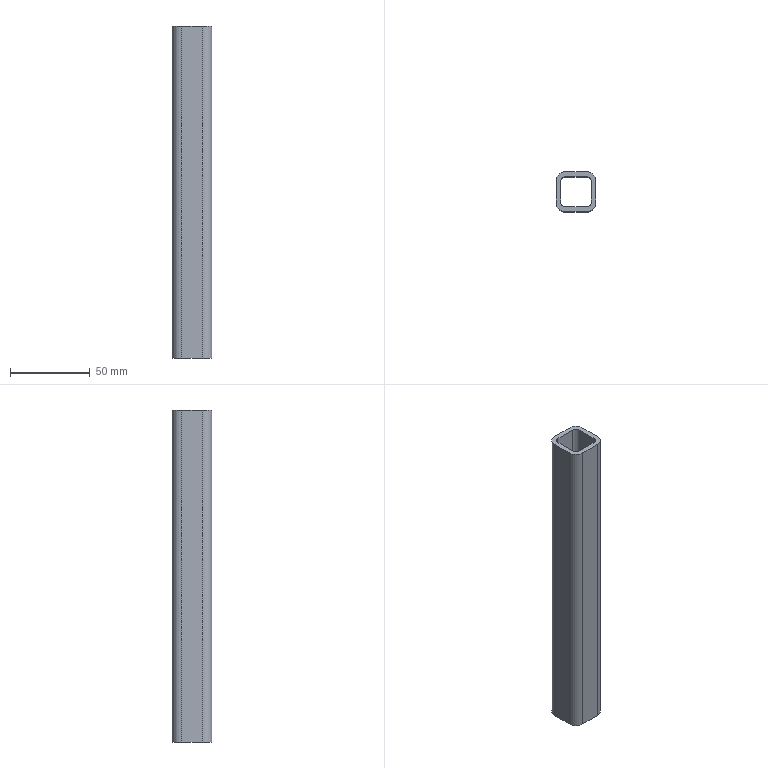Part | STEP file | ISO 10799-2 25x25x3 1784905468712 | 1 solid | 18 faces | box 25 x 25 x 208 mm | volume 50091 mm3 | plane 10 | cylinder 8 | commonest cylinder face diameters 6 x4 12 x4
STEP:
#1=CARTESIAN_POINT('',(-6.5,-9.5,208.));
#2=VERTEX_POINT('',#1);
#3=CARTESIAN_POINT('',(6.5,-9.5,208.));
#4=VERTEX_POINT('',#3);
#5=CARTESIAN_POINT('',(3.25,-9.5,208.));
#6=DIRECTION('',(1.,0.,0.));
#7=VECTOR('',#6,10.);
#8=LINE('',#5,#7);
#9=EDGE_CURVE('',#2,#4,#8,.T.);
#10=ORIENTED_EDGE('',*,*,#9,.T.);
#11=CARTESIAN_POINT('',(6.5,-9.5,0.));
#12=VERTEX_POINT('',#11);
#13=CARTESIAN_POINT('',(6.5,-9.5,0.));
#14=DIRECTION('',(0.,0.,1.));
#15=VECTOR('',#14,10.);
#16=LINE('',#13,#15);
#17=EDGE_CURVE('',#12,#4,#16,.T.);
#18=ORIENTED_EDGE('',*,*,#17,.F.);
#19=CARTESIAN_POINT('',(-6.5,-9.5,0.));
#20=VERTEX_POINT('',#19);
#21=CARTESIAN_POINT('',(3.25,-9.5,0.));
#22=DIRECTION('',(1.,0.,0.));
#23=VECTOR('',#22,10.);
#24=LINE('',#21,#23);
#25=EDGE_CURVE('',#20,#12,#24,.T.);
#26=ORIENTED_EDGE('',*,*,#25,.F.);
#27=CARTESIAN_POINT('',(-6.5,-9.5,0.));
#28=DIRECTION('',(0.,0.,1.));
#29=VECTOR('',#28,10.);
#30=LINE('',#27,#29);
#31=EDGE_CURVE('',#20,#2,#30,.T.);
#32=ORIENTED_EDGE('',*,*,#31,.T.);
#33=EDGE_LOOP('',(#10,#18,#26,#32));
#34=FACE_OUTER_BOUND('',#33,.T.);
#35=CARTESIAN_POINT('',(6.5,-9.5,0.));
#36=DIRECTION('',(0.,-1.,0.));
#37=DIRECTION('',(0.,0.,-1.));
#38=AXIS2_PLACEMENT_3D('',#35,#36,#37);
#39=PLANE('',#38);
#40=ADVANCED_FACE('',(#34),#39,.F.);
#41=CARTESIAN_POINT('',(9.5,-6.5,208.));
#42=VERTEX_POINT('',#41);
#43=CARTESIAN_POINT('',(6.5,-6.5,208.));
#44=DIRECTION('',(0.,0.,1.));
#45=DIRECTION('',(0.,1.,0.));
#46=AXIS2_PLACEMENT_3D('',#43,#44,#45);
#47=CIRCLE('',#46,3.);
#48=EDGE_CURVE('',#4,#42,#47,.T.);
#49=ORIENTED_EDGE('',*,*,#48,.T.);
#50=CARTESIAN_POINT('',(9.5,-6.5,0.));
#51=VERTEX_POINT('',#50);
#52=CARTESIAN_POINT('',(9.5,-6.5,0.));
#53=DIRECTION('',(0.,0.,1.));
#54=VECTOR('',#53,10.);
#55=LINE('',#52,#54);
#56=EDGE_CURVE('',#51,#42,#55,.T.);
#57=ORIENTED_EDGE('',*,*,#56,.F.);
#58=CARTESIAN_POINT('',(6.5,-6.5,0.));
#59=DIRECTION('',(0.,0.,1.));
#60=DIRECTION('',(0.,1.,0.));
#61=AXIS2_PLACEMENT_3D('',#58,#59,#60);
#62=CIRCLE('',#61,3.);
#63=EDGE_CURVE('',#12,#51,#62,.T.);
#64=ORIENTED_EDGE('',*,*,#63,.F.);
#65=ORIENTED_EDGE('',*,*,#17,.T.);
#66=EDGE_LOOP('',(#49,#57,#64,#65));
#67=FACE_OUTER_BOUND('',#66,.T.);
#68=CARTESIAN_POINT('',(6.5,-6.5,0.));
#69=DIRECTION('',(0.,0.,1.));
#70=DIRECTION('',(0.,1.,0.));
#71=AXIS2_PLACEMENT_3D('',#68,#69,#70);
#72=CYLINDRICAL_SURFACE('',#71,3.);
#73=ADVANCED_FACE('',(#67),#72,.F.);
#74=CARTESIAN_POINT('',(9.5,6.5,208.));
#75=VERTEX_POINT('',#74);
#76=CARTESIAN_POINT('',(9.5,3.25,208.));
#77=DIRECTION('',(0.,1.,0.));
#78=VECTOR('',#77,10.);
#79=LINE('',#76,#78);
#80=EDGE_CURVE('',#42,#75,#79,.T.);
#81=ORIENTED_EDGE('',*,*,#80,.T.);
#82=CARTESIAN_POINT('',(9.5,6.5,0.));
#83=VERTEX_POINT('',#82);
#84=CARTESIAN_POINT('',(9.5,6.5,0.));
#85=DIRECTION('',(0.,0.,1.));
#86=VECTOR('',#85,10.);
#87=LINE('',#84,#86);
#88=EDGE_CURVE('',#83,#75,#87,.T.);
#89=ORIENTED_EDGE('',*,*,#88,.F.);
#90=CARTESIAN_POINT('',(9.5,3.25,0.));
#91=DIRECTION('',(0.,1.,0.));
#92=VECTOR('',#91,10.);
#93=LINE('',#90,#92);
#94=EDGE_CURVE('',#51,#83,#93,.T.);
#95=ORIENTED_EDGE('',*,*,#94,.F.);
#96=ORIENTED_EDGE('',*,*,#56,.T.);
#97=EDGE_LOOP('',(#81,#89,#95,#96));
#98=FACE_OUTER_BOUND('',#97,.T.);
#99=CARTESIAN_POINT('',(9.5,6.5,0.));
#100=DIRECTION('',(1.,0.,0.));
#101=DIRECTION('',(0.,0.,-1.));
#102=AXIS2_PLACEMENT_3D('',#99,#100,#101);
#103=PLANE('',#102);
#104=ADVANCED_FACE('',(#98),#103,.F.);
#105=CARTESIAN_POINT('',(6.5,9.5,208.));
#106=VERTEX_POINT('',#105);
#107=CARTESIAN_POINT('',(6.5,6.5,208.));
#108=DIRECTION('',(0.,0.,1.));
#109=DIRECTION('',(-1.,0.,0.));
#110=AXIS2_PLACEMENT_3D('',#107,#108,#109);
#111=CIRCLE('',#110,3.);
#112=EDGE_CURVE('',#75,#106,#111,.T.);
#113=ORIENTED_EDGE('',*,*,#112,.T.);
#114=CARTESIAN_POINT('',(6.5,9.5,0.));
#115=VERTEX_POINT('',#114);
#116=CARTESIAN_POINT('',(6.5,9.5,0.));
#117=DIRECTION('',(0.,0.,1.));
#118=VECTOR('',#117,10.);
#119=LINE('',#116,#118);
#120=EDGE_CURVE('',#115,#106,#119,.T.);
#121=ORIENTED_EDGE('',*,*,#120,.F.);
#122=CARTESIAN_POINT('',(6.5,6.5,0.));
#123=DIRECTION('',(0.,0.,1.));
#124=DIRECTION('',(-1.,0.,0.));
#125=AXIS2_PLACEMENT_3D('',#122,#123,#124);
#126=CIRCLE('',#125,3.);
#127=EDGE_CURVE('',#83,#115,#126,.T.);
#128=ORIENTED_EDGE('',*,*,#127,.F.);
#129=ORIENTED_EDGE('',*,*,#88,.T.);
#130=EDGE_LOOP('',(#113,#121,#128,#129));
#131=FACE_OUTER_BOUND('',#130,.T.);
#132=CARTESIAN_POINT('',(6.5,6.5,0.));
#133=DIRECTION('',(0.,0.,1.));
#134=DIRECTION('',(-1.,0.,0.));
#135=AXIS2_PLACEMENT_3D('',#132,#133,#134);
#136=CYLINDRICAL_SURFACE('',#135,3.);
#137=ADVANCED_FACE('',(#131),#136,.F.);
#138=CARTESIAN_POINT('',(12.5,6.5,208.));
#139=VERTEX_POINT('',#138);
#140=CARTESIAN_POINT('',(12.5,-6.5,208.));
#141=VERTEX_POINT('',#140);
#142=CARTESIAN_POINT('',(12.5,3.25,208.));
#143=DIRECTION('',(0.,-1.,0.));
#144=VECTOR('',#143,10.);
#145=LINE('',#142,#144);
#146=EDGE_CURVE('',#139,#141,#145,.T.);
#147=ORIENTED_EDGE('',*,*,#146,.T.);
#148=CARTESIAN_POINT('',(12.5,-6.5,0.));
#149=VERTEX_POINT('',#148);
#150=CARTESIAN_POINT('',(12.5,-6.5,0.));
#151=DIRECTION('',(0.,0.,1.));
#152=VECTOR('',#151,10.);
#153=LINE('',#150,#152);
#154=EDGE_CURVE('',#149,#141,#153,.T.);
#155=ORIENTED_EDGE('',*,*,#154,.F.);
#156=CARTESIAN_POINT('',(12.5,6.5,0.));
#157=VERTEX_POINT('',#156);
#158=CARTESIAN_POINT('',(12.5,3.25,0.));
#159=DIRECTION('',(0.,-1.,0.));
#160=VECTOR('',#159,10.);
#161=LINE('',#158,#160);
#162=EDGE_CURVE('',#157,#149,#161,.T.);
#163=ORIENTED_EDGE('',*,*,#162,.F.);
#164=CARTESIAN_POINT('',(12.5,6.5,0.));
#165=DIRECTION('',(0.,0.,1.));
#166=VECTOR('',#165,10.);
#167=LINE('',#164,#166);
#168=EDGE_CURVE('',#157,#139,#167,.T.);
#169=ORIENTED_EDGE('',*,*,#168,.T.);
#170=EDGE_LOOP('',(#147,#155,#163,#169));
#171=FACE_OUTER_BOUND('',#170,.T.);
#172=CARTESIAN_POINT('',(12.5,6.5,0.));
#173=DIRECTION('',(1.,0.,0.));
#174=DIRECTION('',(0.,0.,-1.));
#175=AXIS2_PLACEMENT_3D('',#172,#173,#174);
#176=PLANE('',#175);
#177=ADVANCED_FACE('',(#171),#176,.T.);
#178=CARTESIAN_POINT('',(6.5,-12.5,208.));
#179=VERTEX_POINT('',#178);
#180=CARTESIAN_POINT('',(6.5,-6.5,208.));
#181=DIRECTION('',(0.,0.,-1.));
#182=DIRECTION('',(0.,1.,0.));
#183=AXIS2_PLACEMENT_3D('',#180,#181,#182);
#184=CIRCLE('',#183,6.);
#185=EDGE_CURVE('',#141,#179,#184,.T.);
#186=ORIENTED_EDGE('',*,*,#185,.T.);
#187=CARTESIAN_POINT('',(6.5,-12.5,0.));
#188=VERTEX_POINT('',#187);
#189=CARTESIAN_POINT('',(6.5,-12.5,0.));
#190=DIRECTION('',(0.,0.,1.));
#191=VECTOR('',#190,10.);
#192=LINE('',#189,#191);
#193=EDGE_CURVE('',#188,#179,#192,.T.);
#194=ORIENTED_EDGE('',*,*,#193,.F.);
#195=CARTESIAN_POINT('',(6.5,-6.5,0.));
#196=DIRECTION('',(0.,0.,-1.));
#197=DIRECTION('',(0.,1.,0.));
#198=AXIS2_PLACEMENT_3D('',#195,#196,#197);
#199=CIRCLE('',#198,6.);
#200=EDGE_CURVE('',#149,#188,#199,.T.);
#201=ORIENTED_EDGE('',*,*,#200,.F.);
#202=ORIENTED_EDGE('',*,*,#154,.T.);
#203=EDGE_LOOP('',(#186,#194,#201,#202));
#204=FACE_OUTER_BOUND('',#203,.T.);
#205=CARTESIAN_POINT('',(6.5,-6.5,0.));
#206=DIRECTION('',(0.,0.,1.));
#207=DIRECTION('',(0.,1.,0.));
#208=AXIS2_PLACEMENT_3D('',#205,#206,#207);
#209=CYLINDRICAL_SURFACE('',#208,6.);
#210=ADVANCED_FACE('',(#204),#209,.T.);
#211=CARTESIAN_POINT('',(-6.5,-12.5,208.));
#212=VERTEX_POINT('',#211);
#213=CARTESIAN_POINT('',(3.25,-12.5,208.));
#214=DIRECTION('',(-1.,0.,0.));
#215=VECTOR('',#214,10.);
#216=LINE('',#213,#215);
#217=EDGE_CURVE('',#179,#212,#216,.T.);
#218=ORIENTED_EDGE('',*,*,#217,.T.);
#219=CARTESIAN_POINT('',(-6.5,-12.5,0.));
#220=VERTEX_POINT('',#219);
#221=CARTESIAN_POINT('',(-6.5,-12.5,0.));
#222=DIRECTION('',(0.,0.,1.));
#223=VECTOR('',#222,10.);
#224=LINE('',#221,#223);
#225=EDGE_CURVE('',#220,#212,#224,.T.);
#226=ORIENTED_EDGE('',*,*,#225,.F.);
#227=CARTESIAN_POINT('',(3.25,-12.5,0.));
#228=DIRECTION('',(-1.,0.,0.));
#229=VECTOR('',#228,10.);
#230=LINE('',#227,#229);
#231=EDGE_CURVE('',#188,#220,#230,.T.);
#232=ORIENTED_EDGE('',*,*,#231,.F.);
#233=ORIENTED_EDGE('',*,*,#193,.T.);
#234=EDGE_LOOP('',(#218,#226,#232,#233));
#235=FACE_OUTER_BOUND('',#234,.T.);
#236=CARTESIAN_POINT('',(6.5,-12.5,0.));
#237=DIRECTION('',(0.,-1.,0.));
#238=DIRECTION('',(0.,0.,-1.));
#239=AXIS2_PLACEMENT_3D('',#236,#237,#238);
#240=PLANE('',#239);
#241=ADVANCED_FACE('',(#235),#240,.T.);
#242=CARTESIAN_POINT('',(-12.5,-6.5,208.));
#243=VERTEX_POINT('',#242);
#244=CARTESIAN_POINT('',(-6.5,-6.5,208.));
#245=DIRECTION('',(0.,0.,-1.));
#246=DIRECTION('',(1.,0.,0.));
#247=AXIS2_PLACEMENT_3D('',#244,#245,#246);
#248=CIRCLE('',#247,6.);
#249=EDGE_CURVE('',#212,#243,#248,.T.);
#250=ORIENTED_EDGE('',*,*,#249,.T.);
#251=CARTESIAN_POINT('',(-12.5,-6.5,0.));
#252=VERTEX_POINT('',#251);
#253=CARTESIAN_POINT('',(-12.5,-6.5,0.));
#254=DIRECTION('',(0.,0.,1.));
#255=VECTOR('',#254,10.);
#256=LINE('',#253,#255);
#257=EDGE_CURVE('',#252,#243,#256,.T.);
#258=ORIENTED_EDGE('',*,*,#257,.F.);
#259=CARTESIAN_POINT('',(-6.5,-6.5,0.));
#260=DIRECTION('',(0.,0.,-1.));
#261=DIRECTION('',(1.,0.,0.));
#262=AXIS2_PLACEMENT_3D('',#259,#260,#261);
#263=CIRCLE('',#262,6.);
#264=EDGE_CURVE('',#220,#252,#263,.T.);
#265=ORIENTED_EDGE('',*,*,#264,.F.);
#266=ORIENTED_EDGE('',*,*,#225,.T.);
#267=EDGE_LOOP('',(#250,#258,#265,#266));
#268=FACE_OUTER_BOUND('',#267,.T.);
#269=CARTESIAN_POINT('',(-6.5,-6.5,0.));
#270=DIRECTION('',(0.,0.,1.));
#271=DIRECTION('',(1.,0.,0.));
#272=AXIS2_PLACEMENT_3D('',#269,#270,#271);
#273=CYLINDRICAL_SURFACE('',#272,6.);
#274=ADVANCED_FACE('',(#268),#273,.T.);
#275=CARTESIAN_POINT('',(-6.5,9.5,208.));
#276=VERTEX_POINT('',#275);
#277=CARTESIAN_POINT('',(-3.25,9.5,208.));
#278=DIRECTION('',(-1.,0.,0.));
#279=VECTOR('',#278,10.);
#280=LINE('',#277,#279);
#281=EDGE_CURVE('',#106,#276,#280,.T.);
#282=ORIENTED_EDGE('',*,*,#281,.T.);
#283=CARTESIAN_POINT('',(-6.5,9.5,0.));
#284=VERTEX_POINT('',#283);
#285=CARTESIAN_POINT('',(-6.5,9.5,0.));
#286=DIRECTION('',(0.,0.,1.));
#287=VECTOR('',#286,10.);
#288=LINE('',#285,#287);
#289=EDGE_CURVE('',#284,#276,#288,.T.);
#290=ORIENTED_EDGE('',*,*,#289,.F.);
#291=CARTESIAN_POINT('',(-3.25,9.5,0.));
#292=DIRECTION('',(-1.,0.,0.));
#293=VECTOR('',#292,10.);
#294=LINE('',#291,#293);
#295=EDGE_CURVE('',#115,#284,#294,.T.);
#296=ORIENTED_EDGE('',*,*,#295,.F.);
#297=ORIENTED_EDGE('',*,*,#120,.T.);
#298=EDGE_LOOP('',(#282,#290,#296,#297));
#299=FACE_OUTER_BOUND('',#298,.T.);
#300=CARTESIAN_POINT('',(-6.5,9.5,0.));
#301=DIRECTION('',(0.,1.,0.));
#302=DIRECTION('',(0.,0.,1.));
#303=AXIS2_PLACEMENT_3D('',#300,#301,#302);
#304=PLANE('',#303);
#305=ADVANCED_FACE('',(#299),#304,.F.);
#306=CARTESIAN_POINT('',(-9.5,-6.5,208.));
#307=VERTEX_POINT('',#306);
#308=CARTESIAN_POINT('',(-6.5,-6.5,208.));
#309=DIRECTION('',(0.,0.,1.));
#310=DIRECTION('',(1.,0.,0.));
#311=AXIS2_PLACEMENT_3D('',#308,#309,#310);
#312=CIRCLE('',#311,3.);
#313=EDGE_CURVE('',#307,#2,#312,.T.);
#314=ORIENTED_EDGE('',*,*,#313,.T.);
#315=ORIENTED_EDGE('',*,*,#31,.F.);
#316=CARTESIAN_POINT('',(-9.5,-6.5,0.));
#317=VERTEX_POINT('',#316);
#318=CARTESIAN_POINT('',(-6.5,-6.5,0.));
#319=DIRECTION('',(0.,0.,1.));
#320=DIRECTION('',(1.,0.,0.));
#321=AXIS2_PLACEMENT_3D('',#318,#319,#320);
#322=CIRCLE('',#321,3.);
#323=EDGE_CURVE('',#317,#20,#322,.T.);
#324=ORIENTED_EDGE('',*,*,#323,.F.);
#325=CARTESIAN_POINT('',(-9.5,-6.5,0.));
#326=DIRECTION('',(0.,0.,1.));
#327=VECTOR('',#326,10.);
#328=LINE('',#325,#327);
#329=EDGE_CURVE('',#317,#307,#328,.T.);
#330=ORIENTED_EDGE('',*,*,#329,.T.);
#331=EDGE_LOOP('',(#314,#315,#324,#330));
#332=FACE_OUTER_BOUND('',#331,.T.);
#333=CARTESIAN_POINT('',(-6.5,-6.5,0.));
#334=DIRECTION('',(0.,0.,1.));
#335=DIRECTION('',(1.,0.,0.));
#336=AXIS2_PLACEMENT_3D('',#333,#334,#335);
#337=CYLINDRICAL_SURFACE('',#336,3.);
#338=ADVANCED_FACE('',(#332),#337,.F.);
#339=CARTESIAN_POINT('',(-9.5,6.5,208.));
#340=VERTEX_POINT('',#339);
#341=CARTESIAN_POINT('',(-9.5,-3.25,208.));
#342=DIRECTION('',(0.,-1.,0.));
#343=VECTOR('',#342,10.);
#344=LINE('',#341,#343);
#345=EDGE_CURVE('',#340,#307,#344,.T.);
#346=ORIENTED_EDGE('',*,*,#345,.T.);
#347=ORIENTED_EDGE('',*,*,#329,.F.);
#348=CARTESIAN_POINT('',(-9.5,6.5,0.));
#349=VERTEX_POINT('',#348);
#350=CARTESIAN_POINT('',(-9.5,-3.25,0.));
#351=DIRECTION('',(0.,-1.,0.));
#352=VECTOR('',#351,10.);
#353=LINE('',#350,#352);
#354=EDGE_CURVE('',#349,#317,#353,.T.);
#355=ORIENTED_EDGE('',*,*,#354,.F.);
#356=CARTESIAN_POINT('',(-9.5,6.5,0.));
#357=DIRECTION('',(0.,0.,1.));
#358=VECTOR('',#357,10.);
#359=LINE('',#356,#358);
#360=EDGE_CURVE('',#349,#340,#359,.T.);
#361=ORIENTED_EDGE('',*,*,#360,.T.);
#362=EDGE_LOOP('',(#346,#347,#355,#361));
#363=FACE_OUTER_BOUND('',#362,.T.);
#364=CARTESIAN_POINT('',(-9.5,-6.5,0.));
#365=DIRECTION('',(-1.,0.,0.));
#366=DIRECTION('',(0.,0.,1.));
#367=AXIS2_PLACEMENT_3D('',#364,#365,#366);
#368=PLANE('',#367);
#369=ADVANCED_FACE('',(#363),#368,.F.);
#370=CARTESIAN_POINT('',(-6.5,6.5,208.));
#371=DIRECTION('',(0.,0.,1.));
#372=DIRECTION('',(0.,-1.,0.));
#373=AXIS2_PLACEMENT_3D('',#370,#371,#372);
#374=CIRCLE('',#373,3.);
#375=EDGE_CURVE('',#276,#340,#374,.T.);
#376=ORIENTED_EDGE('',*,*,#375,.T.);
#377=ORIENTED_EDGE('',*,*,#360,.F.);
#378=CARTESIAN_POINT('',(-6.5,6.5,0.));
#379=DIRECTION('',(0.,0.,1.));
#380=DIRECTION('',(0.,-1.,0.));
#381=AXIS2_PLACEMENT_3D('',#378,#379,#380);
#382=CIRCLE('',#381,3.);
#383=EDGE_CURVE('',#284,#349,#382,.T.);
#384=ORIENTED_EDGE('',*,*,#383,.F.);
#385=ORIENTED_EDGE('',*,*,#289,.T.);
#386=EDGE_LOOP('',(#376,#377,#384,#385));
#387=FACE_OUTER_BOUND('',#386,.T.);
#388=CARTESIAN_POINT('',(-6.5,6.5,0.));
#389=DIRECTION('',(0.,0.,1.));
#390=DIRECTION('',(0.,-1.,0.));
#391=AXIS2_PLACEMENT_3D('',#388,#389,#390);
#392=CYLINDRICAL_SURFACE('',#391,3.);
#393=ADVANCED_FACE('',(#387),#392,.F.);
#394=CARTESIAN_POINT('',(-12.5,6.5,208.));
#395=VERTEX_POINT('',#394);
#396=CARTESIAN_POINT('',(-12.5,-3.25,208.));
#397=DIRECTION('',(0.,1.,0.));
#398=VECTOR('',#397,10.);
#399=LINE('',#396,#398);
#400=EDGE_CURVE('',#243,#395,#399,.T.);
#401=ORIENTED_EDGE('',*,*,#400,.T.);
#402=CARTESIAN_POINT('',(-12.5,6.5,0.));
#403=VERTEX_POINT('',#402);
#404=CARTESIAN_POINT('',(-12.5,6.5,0.));
#405=DIRECTION('',(0.,0.,1.));
#406=VECTOR('',#405,10.);
#407=LINE('',#404,#406);
#408=EDGE_CURVE('',#403,#395,#407,.T.);
#409=ORIENTED_EDGE('',*,*,#408,.F.);
#410=CARTESIAN_POINT('',(-12.5,-3.25,0.));
#411=DIRECTION('',(0.,1.,0.));
#412=VECTOR('',#411,10.);
#413=LINE('',#410,#412);
#414=EDGE_CURVE('',#252,#403,#413,.T.);
#415=ORIENTED_EDGE('',*,*,#414,.F.);
#416=ORIENTED_EDGE('',*,*,#257,.T.);
#417=EDGE_LOOP('',(#401,#409,#415,#416));
#418=FACE_OUTER_BOUND('',#417,.T.);
#419=CARTESIAN_POINT('',(-12.5,-6.5,0.));
#420=DIRECTION('',(-1.,0.,0.));
#421=DIRECTION('',(0.,0.,1.));
#422=AXIS2_PLACEMENT_3D('',#419,#420,#421);
#423=PLANE('',#422);
#424=ADVANCED_FACE('',(#418),#423,.T.);
#425=CARTESIAN_POINT('',(-6.5,12.5,208.));
#426=VERTEX_POINT('',#425);
#427=CARTESIAN_POINT('',(-6.5,6.5,208.));
#428=DIRECTION('',(0.,0.,-1.));
#429=DIRECTION('',(0.,-1.,0.));
#430=AXIS2_PLACEMENT_3D('',#427,#428,#429);
#431=CIRCLE('',#430,6.);
#432=EDGE_CURVE('',#395,#426,#431,.T.);
#433=ORIENTED_EDGE('',*,*,#432,.T.);
#434=CARTESIAN_POINT('',(-6.5,12.5,0.));
#435=VERTEX_POINT('',#434);
#436=CARTESIAN_POINT('',(-6.5,12.5,0.));
#437=DIRECTION('',(0.,0.,1.));
#438=VECTOR('',#437,10.);
#439=LINE('',#436,#438);
#440=EDGE_CURVE('',#435,#426,#439,.T.);
#441=ORIENTED_EDGE('',*,*,#440,.F.);
#442=CARTESIAN_POINT('',(-6.5,6.5,0.));
#443=DIRECTION('',(0.,0.,-1.));
#444=DIRECTION('',(0.,-1.,0.));
#445=AXIS2_PLACEMENT_3D('',#442,#443,#444);
#446=CIRCLE('',#445,6.);
#447=EDGE_CURVE('',#403,#435,#446,.T.);
#448=ORIENTED_EDGE('',*,*,#447,.F.);
#449=ORIENTED_EDGE('',*,*,#408,.T.);
#450=EDGE_LOOP('',(#433,#441,#448,#449));
#451=FACE_OUTER_BOUND('',#450,.T.);
#452=CARTESIAN_POINT('',(-6.5,6.5,0.));
#453=DIRECTION('',(0.,0.,1.));
#454=DIRECTION('',(0.,-1.,0.));
#455=AXIS2_PLACEMENT_3D('',#452,#453,#454);
#456=CYLINDRICAL_SURFACE('',#455,6.);
#457=ADVANCED_FACE('',(#451),#456,.T.);
#458=CARTESIAN_POINT('',(6.5,12.5,208.));
#459=VERTEX_POINT('',#458);
#460=CARTESIAN_POINT('',(-3.25,12.5,208.));
#461=DIRECTION('',(1.,0.,0.));
#462=VECTOR('',#461,10.);
#463=LINE('',#460,#462);
#464=EDGE_CURVE('',#426,#459,#463,.T.);
#465=ORIENTED_EDGE('',*,*,#464,.T.);
#466=CARTESIAN_POINT('',(6.5,12.5,0.));
#467=VERTEX_POINT('',#466);
#468=CARTESIAN_POINT('',(6.5,12.5,0.));
#469=DIRECTION('',(0.,0.,1.));
#470=VECTOR('',#469,10.);
#471=LINE('',#468,#470);
#472=EDGE_CURVE('',#467,#459,#471,.T.);
#473=ORIENTED_EDGE('',*,*,#472,.F.);
#474=CARTESIAN_POINT('',(-3.25,12.5,0.));
#475=DIRECTION('',(1.,0.,0.));
#476=VECTOR('',#475,10.);
#477=LINE('',#474,#476);
#478=EDGE_CURVE('',#435,#467,#477,.T.);
#479=ORIENTED_EDGE('',*,*,#478,.F.);
#480=ORIENTED_EDGE('',*,*,#440,.T.);
#481=EDGE_LOOP('',(#465,#473,#479,#480));
#482=FACE_OUTER_BOUND('',#481,.T.);
#483=CARTESIAN_POINT('',(-6.5,12.5,0.));
#484=DIRECTION('',(0.,1.,0.));
#485=DIRECTION('',(0.,0.,1.));
#486=AXIS2_PLACEMENT_3D('',#483,#484,#485);
#487=PLANE('',#486);
#488=ADVANCED_FACE('',(#482),#487,.T.);
#489=CARTESIAN_POINT('',(6.5,6.5,208.));
#490=DIRECTION('',(0.,0.,-1.));
#491=DIRECTION('',(-1.,0.,0.));
#492=AXIS2_PLACEMENT_3D('',#489,#490,#491);
#493=CIRCLE('',#492,6.);
#494=EDGE_CURVE('',#459,#139,#493,.T.);
#495=ORIENTED_EDGE('',*,*,#494,.T.);
#496=ORIENTED_EDGE('',*,*,#168,.F.);
#497=CARTESIAN_POINT('',(6.5,6.5,0.));
#498=DIRECTION('',(0.,0.,-1.));
#499=DIRECTION('',(-1.,0.,0.));
#500=AXIS2_PLACEMENT_3D('',#497,#498,#499);
#501=CIRCLE('',#500,6.);
#502=EDGE_CURVE('',#467,#157,#501,.T.);
#503=ORIENTED_EDGE('',*,*,#502,.F.);
#504=ORIENTED_EDGE('',*,*,#472,.T.);
#505=EDGE_LOOP('',(#495,#496,#503,#504));
#506=FACE_OUTER_BOUND('',#505,.T.);
#507=CARTESIAN_POINT('',(6.5,6.5,0.));
#508=DIRECTION('',(0.,0.,1.));
#509=DIRECTION('',(-1.,0.,0.));
#510=AXIS2_PLACEMENT_3D('',#507,#508,#509);
#511=CYLINDRICAL_SURFACE('',#510,6.);
#512=ADVANCED_FACE('',(#506),#511,.T.);
#513=ORIENTED_EDGE('',*,*,#414,.T.);
#514=ORIENTED_EDGE('',*,*,#447,.T.);
#515=ORIENTED_EDGE('',*,*,#478,.T.);
#516=ORIENTED_EDGE('',*,*,#502,.T.);
#517=ORIENTED_EDGE('',*,*,#162,.T.);
#518=ORIENTED_EDGE('',*,*,#200,.T.);
#519=ORIENTED_EDGE('',*,*,#231,.T.);
#520=ORIENTED_EDGE('',*,*,#264,.T.);
#521=EDGE_LOOP('',(#513,#514,#515,#516,#517,#518,#519,#520));
#522=FACE_OUTER_BOUND('',#521,.T.);
#523=ORIENTED_EDGE('',*,*,#295,.T.);
#524=ORIENTED_EDGE('',*,*,#383,.T.);
#525=ORIENTED_EDGE('',*,*,#354,.T.);
#526=ORIENTED_EDGE('',*,*,#323,.T.);
#527=ORIENTED_EDGE('',*,*,#25,.T.);
#528=ORIENTED_EDGE('',*,*,#63,.T.);
#529=ORIENTED_EDGE('',*,*,#94,.T.);
#530=ORIENTED_EDGE('',*,*,#127,.T.);
#531=EDGE_LOOP('',(#523,#524,#525,#526,#527,#528,#529,#530));
#532=FACE_BOUND('',#531,.T.);
#533=CARTESIAN_POINT('',(0.,0.,0.));
#534=DIRECTION('',(0.,0.,1.));
#535=DIRECTION('',(1.,0.,0.));
#536=AXIS2_PLACEMENT_3D('',#533,#534,#535);
#537=PLANE('',#536);
#538=ADVANCED_FACE('',(#522,#532),#537,.F.);
#539=ORIENTED_EDGE('',*,*,#400,.F.);
#540=ORIENTED_EDGE('',*,*,#249,.F.);
#541=ORIENTED_EDGE('',*,*,#217,.F.);
#542=ORIENTED_EDGE('',*,*,#185,.F.);
#543=ORIENTED_EDGE('',*,*,#146,.F.);
#544=ORIENTED_EDGE('',*,*,#494,.F.);
#545=ORIENTED_EDGE('',*,*,#464,.F.);
#546=ORIENTED_EDGE('',*,*,#432,.F.);
#547=EDGE_LOOP('',(#539,#540,#541,#542,#543,#544,#545,#546));
#548=FACE_OUTER_BOUND('',#547,.T.);
#549=ORIENTED_EDGE('',*,*,#281,.F.);
#550=ORIENTED_EDGE('',*,*,#112,.F.);
#551=ORIENTED_EDGE('',*,*,#80,.F.);
#552=ORIENTED_EDGE('',*,*,#48,.F.);
#553=ORIENTED_EDGE('',*,*,#9,.F.);
#554=ORIENTED_EDGE('',*,*,#313,.F.);
#555=ORIENTED_EDGE('',*,*,#345,.F.);
#556=ORIENTED_EDGE('',*,*,#375,.F.);
#557=EDGE_LOOP('',(#549,#550,#551,#552,#553,#554,#555,#556));
#558=FACE_BOUND('',#557,.T.);
#559=CARTESIAN_POINT('',(0.,0.,208.));
#560=DIRECTION('',(0.,0.,1.));
#561=DIRECTION('',(1.,0.,0.));
#562=AXIS2_PLACEMENT_3D('',#559,#560,#561);
#563=PLANE('',#562);
#564=ADVANCED_FACE('',(#548,#558),#563,.T.);
#565=CLOSED_SHELL('',(#40,#73,#104,#137,#177,#210,#241,#274,#305,#338,#369,#393,#424,#457,#488,#512,#538,#564));
#566=MANIFOLD_SOLID_BREP('',#565);
#567=(LENGTH_UNIT()NAMED_UNIT(*)SI_UNIT(.MILLI.,.METRE.));
#568=UNCERTAINTY_MEASURE_WITH_UNIT(LENGTH_MEASURE(0.01),#567,'','');
#569=(NAMED_UNIT(*)PLANE_ANGLE_UNIT()SI_UNIT($,.RADIAN.));
#570=(NAMED_UNIT(*)SI_UNIT($,.STERADIAN.)SOLID_ANGLE_UNIT());
#571=(GEOMETRIC_REPRESENTATION_CONTEXT(3)GLOBAL_UNCERTAINTY_ASSIGNED_CONTEXT((#568))GLOBAL_UNIT_ASSIGNED_CONTEXT((#567,#569,#570))REPRESENTATION_CONTEXT('',''));
#572=ADVANCED_BREP_SHAPE_REPRESENTATION('',(#566),#571);